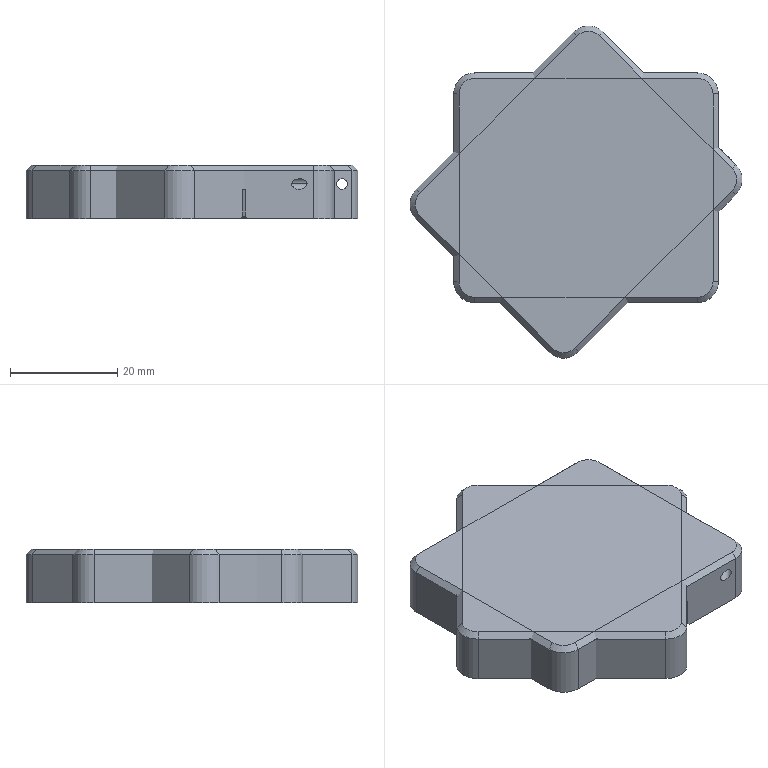NC program | NX | posted with a generic post | part box 61.954 x 61.954 x 10 mm
Lines 1 to 1285 of 3041:
N10 G17 G21 G94 G90
(PLANAR_MILL_5 , TOOL : D50面刀)
N12 T01 M6
N14 G54
N16 G17 G0 G90 X2.65 Y-96.458 B0. C0. S3500 M3
N18 G43 Z30. H1
N20 Z3.
N22 G94 G1 Z0. F800.
N24 Y-46.458
N26 Y41.158
N28 Y91.158
N30 Z3.
N32 G0 Z30.
N34 M5
(ADAPTIVE_MILLING , TOOL : D12开粗)
N36 T02 M6
N38 G54
N40 G17 G0 G90 X45.864 Y7.918 B0. C0. S5500 M3
N42 G43 Z30. H2
N44 Z-9.
N46 G94 G1 X45.758 Y7.813 Z-9.937 F2000.
N48 X45.652 Y7.707 Z-10.308
N50 X45.545 Y7.601 Z-10.58
N52 X45.439 Y7.495 Z-10.8
N54 X45.332 Y7.389 Z-10.984
N56 X45.226 Y7.284 Z-11.142
N58 X45.12 Y7.178 Z-11.28
N60 X45.013 Y7.072 Z-11.4
N62 X44.907 Y6.966 Z-11.505
N64 X44.801 Y6.861 Z-11.598
N66 X44.694 Y6.755 Z-11.679
N68 X44.588 Y6.649 Z-11.75
N70 X44.482 Y6.543 Z-11.81
N72 X44.375 Y6.437 Z-11.862
N74 X44.269 Y6.332 Z-11.905
N76 X44.163 Y6.226 Z-11.939
N78 X44.056 Y6.12 Z-11.966
N80 X43.95 Y6.014 Z-11.985
N82 X43.843 Y5.909 Z-11.996
N84 X43.737 Y5.803 Z-12.
N86 X42.422 Y4.495
N88 G3 X42.184 Y3.112 R1.212
N90 X44.131 Y0.105 R12.601
N92 G2 X45.422 Y-4.633 R6.785
N94 X43.61 Y-9.828 R11.92
N96 X39.648 Y-14.899 R33.153
N98 X31.725 Y-23.034 R288.997
N100 G1 X28.018 Y-26.746
N102 X11.27 Y-43.493
N104 G2 X6.905 Y-45.205 R6.347
N106 X1.737 Y-43.849 R10.676
N108 X-3.181 Y-40.307 R26.17
N110 X-10.332 Y-33.463 R170.745
N112 G1 X-15.854 Y-27.953
N114 X-40.717 Y-3.089
N116 G2 X-42.383 Y1.368 R6.391
N118 X-40.922 Y6.585 R10.897
N120 X-37.309 Y11.506 R27.426
N122 X-29.915 Y19.19 R197.683
N124 G1 X-24.963 Y24.151
N126 X-8.431 Y40.682
N128 G2 X-4.051 Y42.378 R6.371
N130 X1.113 Y41.008 R10.71
N132 X6.085 Y37.411 R26.458
N134 X13.286 Y30.51 R176.153
N136 G1 X19.337 Y24.47
N138 X38.705 Y5.1
N140 G2 X41.867 Y1.252 R35.803
N142 X43.105 Y-5.808 R9.477
N144 X40.632 Y-11.485 R15.987
N146 X36.045 Y-17.112 R45.201
N148 X27.401 Y-25.946 R391.348
N150 G1 X12.916 Y-40.434
N152 G2 X5.632 Y-42.863 R8.751
N154 X-0.237 Y-40.695 R14.363
N156 X-5.656 Y-36.475 R37.421
N158 X-15.223 Y-27.165 R313.101
N160 G1 X-19.574 Y-22.819
N162 X-37.671 Y-4.72
N164 G2 X-40.044 Y2.441 R8.75
N166 X-37.976 Y8.19 R14.179
N168 X-33.635 Y13.804 R36.949
N170 X-25.502 Y22.191 R267.646
N172 G1 X-21.794 Y25.904
N174 X-9.978 Y37.718
N176 G2 X-2.791 Y40.033 R8.762
N178 X2.946 Y37.939 R14.271
N180 X8.488 Y33.644 R36.929
N182 X17.577 Y24.812 R290.323
N184 G1 X21.662 Y20.73
N186 X36.143 Y6.246
N188 G2 X39.473 Y2.465 R34.167
N190 X41.128 Y-6.127 R10.742
N192 X38.425 Y-12.188 R17.777
N194 X33.354 Y-18.384 R50.057
N196 X23.832 Y-28.099 R439.795
N198 G1 X14.435 Y-37.499
N200 G2 X9.94 Y-40.443 R10.989
N202 X3.006 Y-40.323 R11.274
N204 X-2.733 Y-37.26 R20.291
N206 X-8.873 Y-31.967 R63.932
N208 X-20.486 Y-20.491 R824.186
N210 G1 X-34.684 Y-6.293
N212 G2 X-37.66 Y-1.679 R10.928
N214 X-37.454 Y5.255 R11.359
N216 X-34.31 Y11.033 R20.865
N218 X-28.513 Y17.668 R70.416
N220 X-17.842 Y28.442 R844.161
N222 X-10.805 Y35.444 R529.662
N224 X-1.961 Y37.933 R10.223
N226 X4.036 Y35.471 R16.616
N228 X9.946 Y30.78 R43.622
N230 X20.039 Y20.935 R364.834
N232 G1 X24.071 Y16.906
N234 X34.577 Y6.392
N236 G2 X37.549 Y2.972 R27.873
N238 X39.23 Y-6.569 R11.678
N240 X36.346 Y-12.812 R19.439
N242 X31.089 Y-19.22 R53.764
N244 X20.592 Y-29.925 R473.19
N246 X14.471 Y-36.003 R337.67
N248 X4.767 Y-38.917 R11.239
N250 G3 X3.796 Y-39.025 R5.737
N252 G1 X2.351
N254 X0.92 Y-38.819
N256 X-0.467 Y-38.412
N258 X-1.781 Y-37.811
N260 X-2.997 Y-37.029
N262 X-4.089 Y-36.083
N264 X-33.434 Y-6.738
N266 X-34.381 Y-5.646
N268 X-35.162 Y-4.43
N270 G2 X-35.968 Y-2.472 R12.133
N272 X-35.784 Y5.083 R12.762
N274 X-32.538 Y11.24 R21.937
N276 X-26.946 Y17.775 R66.263
N278 X-16.167 Y28.701 R685.961
N280 X-11.466 Y33.337 R159.128
N282 X-1.321 Y35.968 R11.28
N284 X4.953 Y33.189 R18.55
N286 X11.178 Y28.145 R50.002
N288 X20.887 Y18.67 R394.863
N290 G1 X25.716 Y13.846
N292 G2 X33.521 Y6.01 R786.277
N294 X36.613 Y1.834 R17.3
N296 X37.842 Y-2.86 R11.908
N298 G1 X37.927 Y-3.449
N300 Y-4.896
N302 G2 X36.789 Y-9.095 R13.102
N304 X32.768 Y-15.549 R28.888
N306 X25.933 Y-23.096 R104.429
N308 X14.24 Y-34.842 R885.476
N310 X8.976 Y-37.183 R12.835
N312 G3 X7.928 Y-37.812 R6.691
N314 G1 X6.613 Y-38.412
N316 X5.226 Y-38.819
N318 X4.484 Y-38.926
N320 X5.226 Y-38.819
N322 X6.613 Y-38.412
N324 X7.928 Y-37.812
N326 G2 X10.815 Y-36.145 R28.519
N328 G3 X15.297 Y-32.767 R24.971
N330 X20.577 Y-27.655 R178.112
N332 G1 X30.172 Y-18.052
N334 G3 X33.651 Y-13.275 R153.51
N336 G1 X34.722 Y-11.599
N338 G3 X35.932 Y-10.243 R25.584
N340 G1 X36.713 Y-9.028
N342 X37.314 Y-7.713
N344 X37.721 Y-6.326
N346 X37.314 Y-7.713
N348 X36.713 Y-9.028
N350 X35.932 Y-10.243
N352 G2 X34.722 Y-11.599 R25.584
N354 G3 X31.911 Y-14.459 R71.112
N356 G2 X25.581 Y-21.207 R123.303
N358 G1 X15.568 Y-31.237
N360 G2 X13.077 Y-33.244 R60.098
N362 G1 X10.237 Y-36.084
N364 G2 X8.955 Y-37.152 R12.357
N366 G3 X10.237 Y-36.084 R12.357
N368 G1 X34.986 Y-11.335
N370 X35.932 Y-10.243
N372 X36.713 Y-9.028
N374 X37.314 Y-7.713
N376 X37.721 Y-6.326
N378 X37.927 Y-4.896
N380 Y-3.449
N382 X37.722 Y-2.02
N384 X37.315 Y-0.633
N386 X36.714 Y0.682
N388 G3 X32.512 Y6.063 R32.571
N390 X24.435 Y14.277 R397.413
N392 G1 X13.008 Y25.684
N394 G3 X7.413 Y30.564 R117.001
N396 X4.55 Y33.282 R35.895
N398 G1 X3.334 Y34.063
N400 X2.019 Y34.664
N402 X0.632 Y35.071
N404 G3 X-3.491 Y35.413 R21.287
N406 X-10.19 Y33.039 R12.494
N408 X-15.143 Y28.802 R41.357
N410 G1 X-19.309 Y24.695
N412 X-29.488 Y14.51
N414 G3 X-32.611 Y9.971 R131.686
N416 X-34.479 Y6.34 R23.84
N418 G1 X-35.161 Y5.28
N420 X-35.762 Y3.965
N422 X-36.169 Y2.579
N424 X-36.375 Y1.148
N426 Y-0.297
N428 X-36.169 Y-1.728
N430 X-36.375 Y-0.297
N432 Y1.148
N434 X-36.169 Y2.579
N436 X-35.762 Y3.965
N438 X-35.161 Y5.28
N440 X-34.379 Y6.496
N442 G3 X-30.426 Y11.507 R66.
N444 G2 X-25.003 Y17.528 R72.996
N446 X-13.973 Y28.611 R992.035
N448 X-9.717 Y31.882 R30.303
N450 G1 X-8.333 Y32.641
N452 X-7.592 Y33.283
N454 X-6.376 Y34.064
N456 X-5.061 Y34.665
N458 X-3.674 Y35.072
N460 X-2.244 Y35.277
N462 X-0.798
N464 X-2.244
N466 X-3.674 Y35.072
N468 X-5.061 Y34.665
N470 X-6.376 Y34.064
N472 X-7.592 Y33.283
N474 G2 X-12.244 Y29.273 R504.034
N476 G3 X-19.165 Y22.563 R198.313
N478 G1 X-27.806 Y13.915
N480 X-30.109 Y10.912
N482 X-33.433 Y7.588
N484 X-8.685 Y32.336
N486 X-7.592 Y33.283
N488 X-6.376 Y34.064
N490 X-5.061 Y34.665
N492 X-3.674 Y35.072
N494 X-2.244 Y35.277
N496 X-0.798
N498 X0.632 Y35.071
N500 X2.019 Y34.664
N502 X3.334 Y34.063
N504 X4.55 Y33.282
N506 G2 X7.413 Y30.564 R35.895
N508 G1 X34.986 Y2.991
N510 X35.933 Y1.898
N512 G3 X37.991 Y3.023 R1.2
N514 G1 X37.868 Y3.322 Z-11.986
N516 X37.727 Y3.613 Z-11.973
N518 X36.988 Y5.163 Z-11.9
N520 X36.168 Y6.886 F15000.
N522 X36.064 Y7.061
N524 X35.933 Y7.218
N526 X7.717 Y35.434
N528 G3 X5.363 Y37.165 R9.703
N530 X1.49 Y38.546 R15.232
N532 X-1.233 Y38.895 R15.249
N534 X-3.186 Y38.768 R11.294
N536 X-4.871 Y38.466 R19.01
N538 X-8.004 Y37.174 R11.238
N540 X-11.524 Y34.523 R21.466
N542 G1 X-36.548 Y11.28
N544 G3 X-39.506 Y5.358 R9.424
N546 G1 X-39.875 Y1.842
N548 G3 X-39.351 Y0.72 R1.203
N550 G1 X-37.431 Y-0.661 Z-12. F2000.
N552 X-36.564 Y-1.284
N554 G2 X-36.113 Y-1.921 R1.206
N556 G1 X-35.762 Y-3.115
N558 G2 X-36.22 Y-4.442 R1.212
N560 G1 X-37.868 Y-5.62
N562 X-37.99 Y-5.707 Z-11.996
N564 X-38.112 Y-5.794 Z-11.985
N566 X-38.234 Y-5.882 Z-11.966
N568 X-38.356 Y-5.969 Z-11.939
N570 X-38.478 Y-6.056 Z-11.905
N572 X-38.6 Y-6.143 Z-11.862
N574 X-38.722 Y-6.231 Z-11.81
N576 X-38.844 Y-6.318 Z-11.75
N578 X-38.966 Y-6.405 Z-11.679
N580 X-39.088 Y-6.492 Z-11.598
N582 X-39.21 Y-6.58 Z-11.505
N584 X-39.332 Y-6.667 Z-11.4
N586 X-39.454 Y-6.754 Z-11.28
N588 X-39.576 Y-6.841 Z-11.142
N590 X-39.698 Y-6.929 Z-10.984
N592 X-39.82 Y-7.016 Z-10.8
N594 X-39.942 Y-7.103 Z-10.58
N596 X-40.064 Y-7.19 Z-10.308
N598 X-40.186 Y-7.278 Z-9.937
N600 X-40.308 Y-7.365 Z-9.
N602 G0 Z30.
N604 X17.764 Y28.59
N606 Z-2.299
N608 G1 X17.675 Y28.469 Z-3.236
N610 X17.586 Y28.349 Z-3.607
N612 X17.496 Y28.228 Z-3.879
N614 X17.407 Y28.108 Z-4.099
N616 X17.318 Y27.987 Z-4.283
N618 X17.228 Y27.867 Z-4.441
N620 X17.139 Y27.746 Z-4.579
N622 X17.049 Y27.626 Z-4.699
N624 X16.96 Y27.505 Z-4.804
N626 X16.871 Y27.385 Z-4.897
N628 X16.781 Y27.264 Z-4.978
N630 X16.692 Y27.144 Z-5.049
N632 X16.603 Y27.023 Z-5.109
N634 X16.513 Y26.903 Z-5.161
N636 X16.424 Y26.782 Z-5.204
N638 X16.335 Y26.662 Z-5.238
N640 X16.245 Y26.541 Z-5.265
N642 X16.156 Y26.421 Z-5.284
N644 X16.067 Y26.3 Z-5.295
N646 X15.977 Y26.18 Z-5.299
N648 X14.794 Y24.584
N650 G3 X14.83 Y23.093 R1.212
N652 G2 X15.676 Y21.855 R4.614
N654 G3 X18.447 Y18.34 R24.192
N656 X22.883 Y13.72 R169.017
N658 G1 X23.232 Y13.522
N660 X24.031 Y13.279
N662 X25.103 Y12.706
N664 X25.798 Y12.135
N666 X25.103 Y12.706
N668 X24.031 Y13.279
N670 G2 X22.838 Y13.682 R6.733
N672 X19.909 Y16.077 R16.483
N674 X16.369 Y20.027 R32.455
N676 X15.93 Y21.378 R11.695
N678 G1 X15.648 Y21.907
N680 X15.93 Y21.378
N682 G2 X16.4 Y19.725 R32.871
N684 G3 X18.265 Y16.767 R10.703
N686 X21.238 Y13.913 R16.259
N688 X21.69 Y13.749 R2.53
N690 G1 X22.868 Y13.632
N692 X23.155 Y13.545
N694 X22.868 Y13.632
N696 X21.509 Y13.762
N698 G2 X19.624 Y14.863 R5.435
N700 X16.481 Y18.68 R12.072
N702 X16.387 Y19.16 R2.728
N704 G1 X16.284 Y20.205
N706 G2 X16.422 Y18.518 R45.121
N708 G3 X17.904 Y15.716 R6.692
N710 X20.237 Y13.753 R7.366
N712 X20.751 Y13.663 R2.06
N714 G1 X21.659 Y13.752
N716 X20.527 Y13.645
N718 G2 X18.769 Y14.471 R3.705
N720 X16.341 Y17.786 R6.934
N722 X16.393 Y18.918 R4.218
N724 G3 X16.302 Y17.432 R7.494
N726 X18.067 Y14.405 R5.347
N728 X19.575 Y13.506 R3.537
N730 X20.449 Y13.633 R1.732
N732 G1 X20.673 Y13.655
N734 G3 X19.806 Y13.451 R4.907
N736 G2 X18.201 Y14.035 R2.725
N738 X16.152 Y17.027 R4.941
N740 X16.282 Y17.796 R1.819
N742 G3 X16.34 Y15.655 R2.573
N744 X18.688 Y13.321 R4.291
N746 X19.355 Y13.301 R1.488
N748 G1 X20.001 Y13.497
N750 X19.141 Y13.241
N752 G2 X17.686 Y13.684 R2.253
N754 X15.924 Y16.376 R3.91
N756 X16.112 Y17.236 R2.439
N758 G3 X15.836 Y16.236 R5.104
N760 X17.222 Y13.562 R3.388
N762 X18.541 Y13.024 R2.154
N764 X19.286 Y13.28 R1.632
N766 G2 X18.455 Y12.966 R1.734
N768 X16.531 Y13.965 R2.763
N770 X15.685 Y15.946 R2.989
N772 X15.929 Y16.633 R1.643
N774 G3 X15.586 Y15.863 R2.49
N776 X16.613 Y13.419 R2.907
N778 X18.011 Y12.763 R2.244
N780 X18.993 Y13.124 R2.099
N782 G2 X18.186 Y12.729 R5.901
N784 X16.567 Y13.256 R2.14
N786 X15.426 Y15.484 R2.835
N788 X15.719 Y16.24 R1.883
N790 G3 X15.326 Y15.433 R5.597
N792 X16.549 Y12.886 R2.701
N794 X17.943 Y12.581 R1.575
N796 G1 X18.151 Y12.667
N798 G3 X18.548 Y14.481 R1.32
N800 G1 X17.715 Y15.795
N802 G3 X15.436 Y15.711 R1.32
N804 X15.322 Y13.98 R1.852
N806 X17.09 Y12.341 R2.567
N808 X18.019 Y12.551 R1.318
N810 X18.279 Y14.418 R1.32
N812 G1 X17.422 Y15.53
N814 G3 X15.356 Y15.561 R1.32
N816 X15.016 Y14.318 R1.454
N818 X16.824 Y12.157 R2.54
N820 X17.82 Y12.384 R1.303
N822 G2 X18.478 Y12.849 R2.462
N824 G3 X17.643 Y12.246 R4.084
N826 G2 X16.426 Y12.192 R1.29
N828 X14.879 Y14.732 R2.514
N830 X15.295 Y15.486 R1.557
N832 G3 X14.803 Y14.827 R4.353
N834 X15.531 Y12.436 R2.329
N836 X16.879 Y11.884 R1.811
N838 X17.792 Y12.362 R1.578
N840 G2 X17.126 Y11.881 R3.209
N842 X15.487 Y12.301 R1.779
N844 X14.588 Y14.381 R2.364
N846 X15.002 Y15.13 R1.556
N848 G3 X14.481 Y14.33 R2.158
N850 X16.352 Y11.626 R2.31
N852 X17.257 Y11.92 R1.32
N854 X17.447 Y13.534 R1.32
N856 G1 X16.817 Y14.572
N858 G3 X14.669 Y14.724 R1.32
N860 X14.329 Y13.218 R1.579
N862 X16.111 Y11.438 R2.305
N864 X17.274 Y11.936 R1.337
N866 G1 X17.448 Y12.079
N868 G2 X16.797 Y11.508 R15.63
N870 X15.426 Y11.571 R1.467
N872 X14.172 Y13.93 R2.314
N874 X14.585 Y14.622 R1.39
N876 G3 X14.056 Y12.887 R1.567
N878 X15.909 Y11.171 R2.271
N880 X17.037 Y11.7 R1.37
N882 G2 X16.473 Y11.211 R2.825
N884 X14.811 Y11.514 R1.703
N886 X13.893 Y13.68 R2.238
N888 X14.329 Y14.366 R1.435
N890 G3 X13.745 Y13.53 R1.691
N892 X15.696 Y10.9 R2.249
N894 X16.775 Y11.438 R1.391
N896 G2 X16.212 Y10.946 R2.963
N898 X14.552 Y11.23 R1.708
N900 X13.602 Y13.368 R2.229
N902 X14.05 Y14.087 R1.426
N904 G3 X13.482 Y13.318 R1.765
N906 X15.416 Y10.631 R2.246
N908 X16.51 Y11.173 R1.397
N910 G2 X15.949 Y10.68 R3.084
N912 X14.426 Y10.86 R1.654
N914 X13.307 Y13.022 R2.282
N916 X13.766 Y13.803 R1.395
N918 G3 X13.202 Y13.073 R2.01
N920 X15.168 Y10.358 R2.251
N922 X16.281 Y10.944 R1.505
N924 G2 X15.664 Y10.401 R3.089
N926 X14.151 Y10.587 R1.665
N928 X13.036 Y12.779 R2.246
N930 X13.497 Y13.534 R1.417
N932 G3 X12.906 Y12.707 R1.751
N934 X14.87 Y10.087 R2.262
N936 X15.966 Y10.629 R1.398
N938 G2 X15.405 Y10.136 R3.101
N940 X13.699 Y10.432 R1.745
N942 X12.771 Y12.55 R2.188
N944 X13.21 Y13.247 R1.43
N946 G3 X12.623 Y12.403 R1.686
N948 X14.622 Y9.811 R2.256
N950 X15.733 Y10.396 R1.504
N952 G2 X15.116 Y9.854 R3.081
N954 X13.432 Y10.151 R1.749
N956 X12.486 Y12.233 R2.215
N958 X12.896 Y12.933 R1.381
N960 G3 X12.399 Y11.195 R1.527
N962 X14.341 Y9.536 R2.261
N964 X15.46 Y10.123 R1.506
N966 G2 X14.844 Y9.58 R3.129
N968 X13.164 Y9.871 R1.746
N970 X12.217 Y11.979 R2.203
N972 X12.669 Y12.706 R1.426
N974 G3 X12.081 Y11.882 R1.742
N976 X14.042 Y9.262 R2.263
N978 X15.143 Y9.806 R1.4
N980 G2 X14.582 Y9.312 R3.142
N982 X13.214 Y9.401 R1.565
N984 X11.918 Y11.617 R2.292
N986 X12.389 Y12.426 R1.395
N988 G3 X11.804 Y11.603 R1.712
N990 X13.779 Y8.985 R2.267
N992 X14.86 Y9.523 R1.392
N994 G2 X14.298 Y9.032 R2.987
N996 X12.609 Y9.326 R1.74
N998 X11.643 Y11.338 R2.272
N1000 X12.116 Y12.153 R1.395
N1002 G3 X11.529 Y11.323 R1.714
N1004 X13.5 Y8.712 R2.267
N1006 X14.642 Y9.305 R1.512
N1008 G2 X14.027 Y8.759 R3.289
N1010 X12.339 Y9.047 R1.738
N1012 X11.389 Y11.148 R2.201
N1014 X11.843 Y11.881 R1.425
N1016 G3 X11.256 Y11.051 R1.721
N1018 X13.242 Y8.44 R2.255
N1020 X14.365 Y9.028 R1.507
N1022 G2 X13.749 Y8.485 R3.148
N1024 X12.053 Y8.783 R1.748
N1026 X11.121 Y10.899 R2.187
N1028 X11.562 Y11.599 R1.429
N1030 G3 X10.974 Y10.753 R1.689
N1032 X12.973 Y8.164 R2.258
N1034 X14.086 Y8.749 R1.505
N1036 G2 X13.469 Y8.207 R3.09
N1038 X11.782 Y8.504 R1.75
N1040 X10.837 Y10.584 R2.213
N1042 X11.247 Y11.284 R1.381
N1044 G3 X10.75 Y9.546 R1.526
N1046 X12.7 Y7.889 R2.256
N1048 X13.811 Y8.474 R1.504
N1050 G2 X13.182 Y7.926 R2.931
N1052 X11.493 Y8.24 R1.769
N1054 X10.564 Y10.325 R2.21
N1056 X11.018 Y11.055 R1.426
N1058 G3 X10.471 Y10.381 R2.069
N1060 X11.47 Y7.941 R2.211
N1062 X12.98 Y7.73 R1.564
N1064 X13.483 Y8.146 R1.51
N1066 G2 X11.92 Y7.612 R1.309
N1068 X10.28 Y10.051 R2.285
N1070 X10.795 Y10.832 R1.344
N1072 G3 X10.153 Y10.02 R1.491
N1074 X12.277 Y7.322 R2.275
N1076 X13.377 Y8.016 R1.486
N1078 G2 X12.815 Y7.416 R3.065
N1080 X11.299 Y7.463 R1.63
N1082 X10.003 Y9.85 R2.292
N1084 X10.492 Y10.584 R1.344
N1086 G3 X9.837 Y9.032 R1.452
N1088 X12.011 Y7.025 R2.353
N1090 X13.134 Y7.721 R1.48
N1092 G2 X12.573 Y7.121 R3.079
N1094 X11.059 Y7.158 R1.654
N1096 X9.717 Y9.619 R2.343
N1098 X10.209 Y10.351 R1.347
N1100 G3 X9.545 Y8.738 R1.495
N1102 X11.812 Y6.728 R2.37
N1104 X12.713 Y7.207 R1.297
N1106 X12.666 Y8.52 R1.321
N1108 G1 X11.877 Y9.79
N1110 G3 X9.919 Y10.114 R1.32
N1112 X9.349 Y8.726 R1.454
N1114 X11.614 Y6.502 R2.411
N1116 X12.627 Y7.059 R1.28
N1118 X12.486 Y8.68 R1.32
N1120 G1 X11.442 Y9.798
N1122 G3 X9.855 Y10.061 R1.32
N1124 X9.165 Y8.928 R1.328
N1126 X11.502 Y6.272 R2.455
N1128 X12.54 Y6.885 R1.28
N1130 G2 X12.856 Y7.381 R2.147
N1132 G3 X12.429 Y6.689 R3.579
N1134 G2 X11.23 Y6.197 R1.284
N1136 X9.109 Y9.297 R2.476
N1138 X9.839 Y10.052 R1.353
N1140 G3 X9.043 Y9.433 R1.697
N1142 X9.299 Y7.029 R2.309
N1144 X11.524 Y5.966 R2.389
N1146 X12.539 Y6.882 R1.471
N1148 G2 X12.106 Y6.183 R3.148
N1150 X10.596 Y5.932 R1.639
N1152 X8.765 Y9.107 R2.605
N1154 X9.499 Y9.871 R1.353
N1156 G3 X8.706 Y9.259 R1.715
N1158 X8.949 Y6.758 R2.393
N1160 X11.37 Y5.626 R2.515
N1162 X12.354 Y6.537 R1.485
N1164 G2 X11.919 Y5.834 R3.143
N1166 X10.222 Y5.614 R1.785
N1168 X8.405 Y8.895 R2.726
N1170 X9.157 Y9.688 R1.354
N1172 G3 X8.404 Y9.144 R1.829
N1174 X8.43 Y6.732 R2.378
N1176 X11.165 Y5.254 R2.736
N1178 X12.107 Y6.034 R1.279
N1180 X11.808 Y7.392 R1.321
N1182 G1 X10.104 Y9.143
N1184 G3 X8.783 Y9.488 R1.321
N1186 X7.977 Y8.599 R1.275
N1188 X9.227 Y5.406 R2.87
N1190 X11.381 Y5.082 R2.358
N1192 X12.14 Y6.136 R1.421
N1194 G2 X11.853 Y5.379 R2.984
N1196 X10.431 Y4.841 R1.645
N1198 X7.795 Y8.509 R2.973
N1200 X8.615 Y9.438 R1.35
N1202 X10. Y9.026 R1.32
N1204 G1 X11.756 Y6.954
N1206 G2 X12.012 Y5.717 R1.321
N1208 X11.093 Y4.813 R1.232
N1210 X8.414 Y5.638 R2.733
N1212 X7.712 Y8.708 R2.891
N1214 X8.783 Y9.488 R1.466
N1216 G3 X7.93 Y9.164 R2.71
N1218 X7.293 Y7.297 R2.126
N1220 X10.557 Y4.426 R3.178
N1222 X11.995 Y5.658 R1.45
N1224 G2 X11.707 Y4.889 R3.119
N1226 X10.059 Y4.297 R1.917
N1228 X7.14 Y7.974 R3.266
N1230 X7.964 Y9.229 R1.607
N1232 G1 X8.272 Y9.334
N1234 G3 X7.41 Y8.925 R1.789
N1236 X6.907 Y6.708 R2.487
N1238 X10.423 Y3.982 R3.392
N1240 X11.742 Y4.834 R1.485
N1242 G1 X11.769 Y4.904
N1244 G3 X11.501 Y6.033 R1.321
N1246 G1 X9.244 Y8.778
N1248 G3 X7.841 Y9.203 R1.32
N1250 X6.722 Y8.082 R1.605
N1252 X7.743 Y4.575 R3.374
N1254 X10.787 Y3.74 R3.232
N1256 X11.768 Y4.79 R1.306
N1258 X11.439 Y5.794 R1.322
N1260 G1 X8.834 Y8.715
N1262 G3 X7.62 Y9.136 R1.321
N1264 X6.585 Y8.277 R1.494
N1266 X6.867 Y5.048 R3.274
N1268 X10.386 Y3.323 R3.636
N1270 X11.625 Y4.127 R1.596
N1272 X11.786 Y4.973 R2.23
N1274 G1 X11.874 Y5.26
N1276 G3 X11.71 Y4.261 R4.087
N1278 G2 X10.825 Y3.332 R1.392
N1280 X7.905 Y3.713 R3.238
N1282 X6.13 Y7.482 R3.793
N1284 X6.923 Y8.913 R2.211
N1286 X7.405 Y9.112 R2.037
N1288 X8.609 Y8.668 R1.321
N1290 G1 X11.418 Y5.399
N1292 G2 X11.731 Y4.409 R1.322
N1294 X11.026 Y3.325 R1.293
N1296 X8.265 Y3.29 R3.069
N1298 X5.922 Y7.426 R3.935
N1300 X6.713 Y8.892 R2.242
N1302 X7.62 Y9.136 R1.683
N1304 G3 X6.627 Y8.955 R2.768
N1306 X5.594 Y7.173 R2.444
N1308 X9.684 Y2.614 R4.124
N1310 X11.378 Y3.262 R2.424
N1312 X11.718 Y4.284 R1.553
N1314 G2 X11.615 Y3.543 R6.324
N1316 X10.431 Y2.589 R1.864
N1318 X6.919 Y3.397 R3.802
N1320 X5.442 Y7.469 R4.136
N1322 X6.272 Y8.851 R2.387
N1324 X7.009 Y9.076 R1.473
N1326 G3 X6.091 Y8.851 R1.841
N1328 X5.02 Y6.723 R2.764
N1330 X9.562 Y2.055 R4.46
N1332 X11.393 Y2.821 R2.631
N1334 X11.677 Y3.656 R1.344
N1336 X11.351 Y4.426 R1.326
N1338 G1 X7.681 Y8.591
N1340 G3 X6.561 Y9.032 R1.321
N1342 X5.347 Y8.382 R1.512
N1344 X4.801 Y5.212 R3.626
N1346 X9.562 Y1.655 R4.707
N1348 X11.458 Y2.512 R2.703
N1350 X11.71 Y3.328 R1.348
N1352 G1 X11.674 Y3.838
N1354 G2 X11.716 Y2.955 R13.676
N1356 X10.852 Y1.881 R1.679
N1358 X7.686 Y1.706 R3.789
N1360 X4.45 Y6.651 R4.854
N1362 X5.605 Y8.842 R2.999
N1364 X6.246 Y9.027 R1.475
N1366 X7.224 Y8.594 R1.322
N1368 G1 X7.53 Y8.256
N1370 X9.119 Y6.505 Z-5.199
N1372 X9.149 Y6.471 F15000.
N1374 X10.738 Y4.72 Z-5.299 F2000.
N1376 X11.381 Y4.012
N1378 G2 X11.717 Y3.254 R1.326
N1380 X11.261 Y2.054 R1.325
N1382 X8.624 Y1.267 R3.326
N1384 X4.215 Y6.668 R4.991
N1386 X5.358 Y8.838 R3.065
N1388 X6.41 Y9.017 R1.43
N1390 G3 X5.464 Y9.008 R2.143
N1392 X4.093 Y7.52 R2.537
N1394 X4.716 Y3.132 R4.762
N1396 X9.417 Y0.843 R5.119
N1398 X11.577 Y1.97 R3.056
N1400 X11.728 Y3.139 R1.692
N1402 G2 X11.776 Y2.317 R5.515
N1404 X10.636 Y1.027 R2.113
N1406 X6.805 Y1.039 R4.432
N1408 X3.595 Y6.548 R5.392
N1410 X4.935 Y8.903 R3.306
N1412 X5.949 Y9.063 R1.435
N1414 G3 X5.127 Y9.102 R3.999
N1416 X3.542 Y7.596 R2.628
N1418 X3.827 Y3.164 R4.996
N1420 X8.884 Y0.146 R5.659
N1422 X11.565 Y1.32 R3.618
N1424 X11.835 Y2.375 R1.289
N1426 X11.516 Y2.991 R1.332
N1428 G1 X10.549 Y4.042
N1430 X8.948 Y5.782 Z-5.199
N1432 X8.468 Y6.303 F15000.
N1434 X6.867 Y8.043 Z-5.299 F2000.
N1436 X6.516 Y8.43
N1438 X6.153 Y8.805
N1440 G3 X5.426 Y9.114 R1.327
N1442 X4.041 Y8.696 R1.615
N1444 X2.74 Y5.781 R3.933
N1446 X8.832 Y-0.326 R6.008
N1448 X11.485 Y0.729 R3.965
N1450 X11.935 Y2.062 R1.422
N1452 G1 X11.779 Y2.628
N1454 G2 X12.012 Y1.696 R11.41
N1456 X11.295 Y0.375 R1.893
N1458 X8.023 Y-0.55 R4.354
N1460 X2.467 Y5.754 R6.209
N1462 X3.741 Y8.693 R4.159
N1464 X5.024 Y9.177 R1.615
N1466 G1 X5.098 Y9.166
N1468 G2 X5.743 Y8.789 R1.329
N1470 G1 X6.53 Y7.954
N1472 X8.151 Y6.232 Z-5.199
N1474 X8.873 Y5.466 F15000.
N1476 X10.494 Y3.744 Z-5.299 F2000.
N1478 X11.655 Y2.512
N1480 G2 X11.957 Y1.99 R1.341
N1482 X11.783 Y0.771 R1.329
N1484 X9.448 Y-0.714 R3.54
N1486 X4.322 Y0.806 R5.963
N1488 X2.269 Y6.418 R6.177
N1490 X3.716 Y8.925 R3.983
N1492 X5.201 Y9.136 R1.444
N1494 G3 X4.253 Y9.309 R2.089
N1496 X2.463 Y7.96 R2.806
N1498 X2.019 Y3.438 R5.446
N1500 X8.497 Y-1.317 R6.732
N1502 X11.589 Y-0.061 R4.446
N1504 X12.164 Y1.14 R1.753
N1506 X11.997 Y1.857 R2.778
N1508 G1 X12.207 Y1.099
N1510 G2 X11.56 Y-0.299 R2.05
N1512 X8.178 Y-1.584 R4.636
N1514 X1.446 Y5.542 R6.923
N1516 X2.908 Y8.831 R4.663
N1518 X4.234 Y9.394 R1.955
N1520 X4.743 Y9.275 R3.973
N1522 G3 X3.946 Y9.477 R4.312
N1524 X2.143 Y8.473 R2.697
N1526 X0.998 Y4.399 R5.344
N1528 X8.163 Y-2.105 R7.322
N1530 X11.708 Y-0.724 R4.939
N1532 X12.38 Y0.577 R2.151
N1534 X12.138 Y1.391 R1.486
N1536 G2 X12.436 Y0.586 R1.658
N1538 X11.522 Y-1.142 R2.547
N1540 X7.723 Y-2.378 R5.272
N1542 X0.663 Y5.243 R7.525
N1544 X2.249 Y8.909 R5.114
N1546 X3.561 Y9.557 R2.372
N1548 X4.007 Y9.505 R5.03
N1550 X4.547 Y8.972 R1.206
N1552 G1 X4.943 Y8.194
N1554 X6.016 Y6.087 Z-5.199
N1556 X6.492 Y5.153 F15000.
N1558 X6.573 Y5.021
N1560 X6.667 Y4.897
N1562 X7.689 Y3.754
N1564 G3 X8.044 Y3.482 R1.272
N1566 G1 X8.757 Y3.123
N1568 X10.869 Y2.058 Z-5.299 F2000.
N1570 X11.391 Y1.799
N1572 X11.906 Y1.526
N1574 G2 X12.297 Y1.094 R1.218
N1576 X12.373 Y-0.147 R1.377
N1578 X10.292 Y-2.184 R3.739
N1580 X5.095 Y-2.074 R6.565
N1582 X0.352 Y5.179 R7.762
N1584 X1.856 Y8.868 R5.393
N1586 X3.364 Y9.659 R2.507
N1588 X3.878 Y9.568 R2.
N1590 X4.489 Y8.994 R1.204
N1592 G1 X4.874 Y8.216
N1594 X5.923 Y6.097 Z-5.199
N1596 X6.349 Y5.237 F15000.
N1598 X6.435 Y5.093
N1600 X6.538 Y4.961
N1602 X7.76 Y3.622
N1604 G3 X8.105 Y3.359 R1.283
N1606 G1 X8.766 Y3.025
N1608 X10.877 Y1.959 Z-5.299 F2000.
N1610 X11.431 Y1.683
N1612 X11.977 Y1.393
N1614 G2 X12.368 Y0.961 R1.218
N1616 X12.457 Y-0.222 R1.429
N1618 X10.639 Y-2.272 R3.64
N1620 X5.627 Y-2.609 R6.452
N1622 X0.034 Y5.028 R8.012
N1624 X1.584 Y8.945 R5.634
N1626 X3.128 Y9.768 R2.677
N1628 X4.038 Y9.49 R1.563
N1630 G1 X4.253 Y9.424
N1632 G2 X3.462 Y9.793 R3.73
N1634 G3 X2.054 Y9.619 R1.801
N1636 X-0.075 Y7.061 R4.588
N1638 X0.389 Y1.151 R7.451
N1640 X7.781 Y-3.511 R8.361
N1642 X11.836 Y-1.966 R5.795
N1644 X12.782 Y-0.214 R3.097
N1646 X12.669 Y0.397 R1.569
N1648 G1 X12.422 Y0.861
N1650 X12.801 Y0.113
N1652 G2 X12.385 Y-1.573 R2.296
N1654 X9.283 Y-3.618 R5.085
N1656 X2.972 Y-2.321 R7.911
N1658 X-0.795 Y5.164 R8.559
N1660 X0.925 Y9.112 R5.941
N1662 X2.801 Y10.001 R2.954
N1664 X3.573 Y9.738 R1.628
N1666 G3 X2.831 Y10.094 R4.793
N1668 X0.789 Y9.436 R2.794
N1670 X-1.256 Y5.716 R5.808
N1672 X1.362 Y-1.774 R8.748
N1674 X8.634 Y-4.313 R8.692
N1676 X12.388 Y-2.317 R5.85
N1678 X13.112 Y-0.553 R2.894
N1680 X12.711 Y0.319 R1.407
N1682 G2 X13.165 Y-0.466 R1.544
N1684 X12.487 Y-2.509 R2.896
N1686 X8.868 Y-4.582 R5.872
N1688 X1.829 Y-2.669 R8.783
N1690 X-1.67 Y5.004 R9.195
N1692 X0.095 Y9.175 R6.479
N1694 X2.25 Y10.268 R3.543
N1696 X2.898 Y10.108 R1.515
N1698 X3.445 Y9.105 R1.201
N1700 X3.313 Y8.543 Z-5.274 R1.388
N1702 G1 X2.637 Y6.893 Z-5.199
N1704 X2.48 Y6.516 F15000.
N1706 X2.337 Y6.134
N1708 G3 X2.898 Y4.787 R1.2
N1710 X3.41 Y4.543 R2.014
N1712 X4.809 Y6.19 R1.205
N1714 G1 X4.006 Y8.414 Z-5.299 F2000.
N1716 X3.817 Y8.945
N1718 X3.614 Y9.47
N1720 G3 X3.11 Y9.986 R1.208
N1722 G2 X2.728 Y10.244 R7.214
N1724 G3 X1.172 Y10.244 R2.036
N1726 X-1.363 Y7.935 R4.839
N1728 X-1.904 Y1.853 R8.098
N1730 X7.169 Y-5.31 R9.856
N1732 X12.104 Y-3.635 R7.114
N1734 X13.49 Y-1.153 R3.932
N1736 X13.246 Y-0.333 R1.347
N1738 G1 X12.913 Y0.073
N1740 G2 X13.46 Y-0.64 R7.066
N1742 X13.304 Y-2.365 R2.316
N1744 X10.533 Y-4.97 R5.388
N1746 X4.039 Y-5.054 R8.597
N1748 X-2.598 Y3.95 R10.147
N1750 X-1.019 Y8.977 R7.433
N1752 X1.537 Y10.544 R4.224
N1754 X2.881 Y10.133 R1.459
N1756 G3 X2.221 Y10.624 R4.376
N1758 X0.14 Y10.386 R2.766
N1760 X-2.553 Y7.353 R5.796
N1762 X-2.437 Y0.382 R9.156
N1764 X7.007 Y-6.263 R10.621
N1766 X12.244 Y-4.54 R7.822
N1768 X13.853 Y-1.972 R4.564
N1770 X13.482 Y-0.622 R1.374
N1772 G1 X13.292 Y-0.39
N1774 X13.819 Y-1.002
N1776 G2 X13.865 Y-2.538 R2.158
N1778 X11.602 Y-5.36 R5.21
N1780 X5.411 Y-6.461 R8.664
N1782 X-3.543 Y3.718 R10.933
N1784 X-1.956 Y9.014 R8.122
N1786 X0.944 Y10.887 R4.804
N1788 X2.504 Y10.442 R1.65
N1790 G3 X1.839 Y10.956 R14.361
N1792 X-0.382 Y10.793 R2.913
N1794 X-3.314 Y7.762 R6.114
N1796 X-3.603 Y0.601 R9.63
N1798 X6.596 Y-7.238 R11.469
N1800 X12.369 Y-5.501 R8.63
N1802 X14.274 Y-2.629 R5.136
N1804 X14.136 Y-1.317 R1.734
N1806 X13.584 Y-0.723 R5.636
N1808 G1 X14.21 Y-1.369
N1810 G2 X14.376 Y-2.875 R2.114
N1812 X12.435 Y-5.814 R5.228
N1814 X6.44 Y-7.595 R8.868
N1816 X-4.518 Y3.453 R11.741
N1818 X-2.794 Y9.234 R8.793
N1820 X0.21 Y11.242 R5.313
N1822 X1.597 Y11.169 R2.239
N1824 X2.027 Y10.833 R1.936
N1826 G3 X1.329 Y11.387 R1.946
N1828 X-1.096 Y11.159 R3.339
N1830 X-4.215 Y7.947 R6.63
N1832 X-4.724 Y0.711 R10.231
N1834 X6.434 Y-8.253 R12.328
N1836 X12.643 Y-6.385 R9.354
N1838 X14.735 Y-3.268 R5.614
N1840 X14.707 Y-1.969 R2.18
N1842 X14.07 Y-1.21 R2.724
N1844 G1 X14.695 Y-1.856
N1846 G2 X14.841 Y-3.573 R2.411
N1848 X12.705 Y-6.719 R5.779
N1850 X6.427 Y-8.628 R9.552
N1852 X-5.524 Y3.233 R12.604
N1854 X-3.716 Y9.411 R9.512
N1856 X-0.582 Y11.619 R5.937
N1858 X1.161 Y11.594 R2.78
N1860 X1.738 Y11.122 R2.056
N1862 G1 X1.144 Y11.693
N1864 G3 X-0.879 Y11.882 R2.871
N1866 X-4.344 Y9.454 R6.166
N1868 X-6.154 Y2.877 R10.
N1870 X6.486 Y-9.303 R13.173
N1872 X12.953 Y-7.284 R10.051
N1874 X15.218 Y-3.977 R6.214
N1876 X15.23 Y-2.517 R2.594
N1878 X14.996 Y-2.135 R3.506
N1880 G1 X14.518 Y-1.658
N1882 X15.197 Y-2.356
N1884 G2 X15.371 Y-4.117 R2.529
N1886 X13.18 Y-7.503 R6.145
N1888 X6.699 Y-9.69 R10.155
N1890 X-4.328 Y-3.651 R13.441
N1892 X-6.398 Y5.496 R12.639
N1894 X-3.698 Y10.675 R9.134
N1896 X-0.433 Y12.196 R5.485
N1898 X0.855 Y11.966 R2.172
N1900 X1.334 Y11.526 R5.999
N1902 G1 X0.686 Y12.15
N1904 G3 X-1.531 Y12.351 R3.088
N1906 X-5.149 Y9.876 R6.591
N1908 X-7.222 Y3.036 R10.599
N1910 X-0.668 Y-8.198 R14.01
N1912 X8.988 Y-10.141 R13.232
N1914 X14.483 Y-7.042 R9.593
N1916 X15.862 Y-3.727 R5.454
N1918 X15.529 Y-2.668 R1.454
N1920 G1 X15.052 Y-2.191
N1922 X15.731 Y-2.889
N1924 G2 X15.936 Y-4.633 R2.622
N1926 X13.831 Y-8.165 R6.409
N1928 X7.446 Y-10.738 R10.581
N1930 X-3.426 Y-6.515 R14.107
N1932 X-7.605 Y4.167 R14.011
N1934 X-5.023 Y10.57 R10.41
N1936 X-1.425 Y12.648 R6.434
N1938 X0.245 Y12.519 R3.086
N1940 X0.91 Y11.951 R2.446
N1942 G1 X0.27 Y12.583
N1944 G3 X-1.765 Y12.932 R2.96
N1946 X-5.547 Y10.81 R6.578
N1948 X-8.266 Y4.286 R10.761
N1950 X-4.381 Y-6.559 R14.514
N1952 X7.226 Y-11.45 R14.786
N1954 X13.619 Y-9.151 R11.221
N1956 X16.126 Y-4.72 R14.243
N1958 X16.104 Y-3.321 R1.769
N1960 X15.582 Y-2.722 R3.009
N1962 G2 X16.21 Y-3.497 R2.553
N1964 X16.111 Y-4.759 R1.529
N1966 G1 X15.566 Y-6.126
N1968 G2 X13.569 Y-9.226 R16.323
N1970 X10.468 Y-11.201 R7.147
N1972 X2.173 Y-11.22 R13.308
N1974 X-8.663 Y1.987 R15.479
N1976 X-6.878 Y9.707 R12.111
N1978 X-3.086 Y12.894 R8.017
N1980 X-0.393 Y13.08 R4.28
N1982 X0.35 Y12.51 R1.873
N1984 G3 X-0.391 Y13.187 R4.218
N1986 X-2.156 Y13.443 R2.516
N1988 X-6.331 Y11.083 R13.396
N1990 X-8.974 Y6.455 R9.573
N1992 X-8.128 Y-2.906 R14.332
N1994 X5.47 Y-12.557 R16.106
N1996 X10.66 Y-11.827 R12.308
N1998 X13.234 Y-9.578 R13.787
N2000 G2 X10.213 Y-12.102 R13.082
N2002 X6.566 Y-12.955 R8.573
N2004 X-3.518 Y-9.53 R15.619
N2006 X-9.822 Y2.739 R16.202
N2008 X-8.27 Y9.189 R12.231
N2010 X-6.043 Y11.324 R12.571
N2012 G3 X-8.27 Y9.189 R12.695
N2014 X-10.355 Y4.623 R8.203
N2016 X-8.758 Y-4.307 R15.136
N2018 X4.321 Y-13.585 R17.059
N2020 X6.917 Y-13.618 R11.419
N2022 G1 X7.728 Y-13.363
N2024 X9.409 Y-12.596
N2026 X10.24 Y-12.085
N2028 G2 X6.048 Y-13.841 R12.709
N2030 X1.419 Y-13.394 R11.097
N2032 X-10.782 Y0.723 R17.349
N2034 X-10.636 Y5.258 R13.021
N2036 X-9.333 Y7.753 R13.863
N2038 G1 X-9.967 Y6.721
N2040 G3 X-11.191 Y3.552 R16.169
N2042 X-11.124 Y-1.097 R10.468
N2044 X-4.109 Y-11.517 R17.611
N2046 X1.833 Y-14.257 R16.863
N2048 G1 X2.293 Y-14.29
N2050 G3 X5.961 Y-13.906 R16.323
N2052 G1 X6.536 Y-13.733
N2054 X5.802 Y-13.943
N2056 X3.977 Y-14.233
N2058 X2.25 Y-14.291
N2060 G2 X-0.551 Y-13.829 R11.027
N2062 X-7.075 Y-9.518 R16.321
N2064 X-11.592 Y-0.935 R17.4
N2066 G1 X-11.644 Y-0.159
N2068 G2 X-11.219 Y3.465 R16.259
N2070 G1 X-11.174 Y3.608
N2072 G3 X-11.565 Y1.506 R20.494
N2074 G1 X-11.646 Y-0.218
N2076 G3 X-11.095 Y-3.928 R16.359
N2078 X-9.631 Y-7.311 R16.133
N2080 X-7.41 Y-10.156 R16.05
N2082 X-3.168 Y-13.058 R15.351
N2084 X0.452 Y-14.125 R16.094
N2086 G1 X0.9 Y-14.168
N2088 X0.291 Y-14.099
N2090 G2 X-3.168 Y-13.058 R16.407
N2092 X-7.41 Y-10.156 R15.354
N2094 X-9.802 Y-7.006 R15.475
N2096 X-9.858 Y-5.953 R1.322
N2098 G1 X-9.277 Y-4.393
N2100 X-8.451 Y-2.178 Z-5.199
N2102 X-4.312 Y8.922 F15000.
N2104 X-3.486 Y11.138 Z-5.299 F2000.
N2106 X-2.913 Y12.675
N2108 G2 X-2.156 Y13.443 R1.322
N2110 X-0.392 Y13.252 R1.733
N2112 G1 X-0.18 Y13.04
N2114 G3 X-1.341 Y13.661 R1.595
N2116 X-1.969 Y13.516 R1.833
N2118 X-2.687 Y12.031 R1.212
N2120 G1 X-2.144 Y10.264
N2122 X-2.1 Y10.121 Z-5.295
N2124 X-2.056 Y9.977 Z-5.284
N2126 X-2.012 Y9.834 Z-5.265
N2128 X-1.968 Y9.691 Z-5.238
N2130 X-1.924 Y9.547 Z-5.204
N2132 X-1.879 Y9.404 Z-5.161
N2134 X-1.835 Y9.261 Z-5.109
N2136 X-1.791 Y9.117 Z-5.049
N2138 X-1.747 Y8.974 Z-4.978
N2140 X-1.703 Y8.83 Z-4.897
N2142 X-1.659 Y8.687 Z-4.804
N2144 X-1.615 Y8.544 Z-4.699
N2146 X-1.571 Y8.4 Z-4.579
N2148 X-1.527 Y8.257 Z-4.441
N2150 X-1.483 Y8.113 Z-4.283
N2152 X-1.439 Y7.97 Z-4.099
N2154 X-1.395 Y7.827 Z-3.879
N2156 X-1.351 Y7.683 Z-3.607
N2158 X-1.307 Y7.54 Z-3.236
N2160 X-1.263 Y7.397 Z-2.299
N2162 G0 Z30.
N2164 M5
(ADAPTIVE_MILLING_COPY , TOOL : D6精光)
N2166 T13 M6
N2168 G54
N2170 G17 G0 G90 X-1.295 Y12.102 B0. C0. S5500 M3
N2172 G43 Z30. H13
N2174 Z-2.299
N2176 G94 G1 X-1.204 Y12.221 Z-3.236 F2000.
N2178 X-1.113 Y12.341 Z-3.607
N2180 X-1.022 Y12.46 Z-3.879
N2182 X-0.93 Y12.579 Z-4.099
N2184 X-0.839 Y12.698 Z-4.283
N2186 X-0.748 Y12.817 Z-4.441
N2188 X-0.657 Y12.936 Z-4.579
N2190 X-0.566 Y13.055 Z-4.699
N2192 X-0.474 Y13.174 Z-4.804
N2194 X-0.383 Y13.293 Z-4.897
N2196 X-0.292 Y13.412 Z-4.978
N2198 X-0.201 Y13.531 Z-5.049
N2200 X-0.11 Y13.651 Z-5.109
N2202 X-0.018 Y13.77 Z-5.161
N2204 X0.073 Y13.889 Z-5.204
N2206 X0.164 Y14.008 Z-5.238
N2208 X0.255 Y14.127 Z-5.265
N2210 X0.346 Y14.246 Z-5.284
N2212 X0.438 Y14.365 Z-5.295
N2214 X0.529 Y14.484 Z-5.299
N2216 X1.112 Y15.246
N2218 G3 X1.06 Y16.043 R0.606
N2220 X-0.671 Y16.93 R2.916
N2222 X-1.658 Y16.729 R3.153
N2224 G2 X-0.279 Y16.913 R3.123
N2226 X0.87 Y16.233 R2.13
N2228 G3 X-0.524 Y16.936 R2.001
N2230 X-1.083 Y16.176 R0.606
N2232 G1 X-0.877 Y15.397
N2234 X-0.839 Y15.252 Z-5.295
N2236 X-0.801 Y15.107 Z-5.284
N2238 X-0.763 Y14.962 Z-5.265
N2240 X-0.724 Y14.817 Z-5.238
N2242 X-0.686 Y14.672 Z-5.204
N2244 X-0.648 Y14.527 Z-5.161
N2246 X-0.61 Y14.382 Z-5.109
N2248 X-0.571 Y14.237 Z-5.049
N2250 X-0.533 Y14.092 Z-4.978
N2252 X-0.495 Y13.947 Z-4.897
N2254 X-0.457 Y13.802 Z-4.804
N2256 X-0.418 Y13.657 Z-4.699
N2258 X-0.38 Y13.512 Z-4.579
N2260 X-0.342 Y13.367 Z-4.441
N2262 X-0.304 Y13.222 Z-4.283
N2264 X-0.265 Y13.076 Z-4.099
N2266 X-0.227 Y12.931 Z-3.879
N2268 X-0.189 Y12.786 Z-3.607
N2270 X-0.151 Y12.641 Z-3.236
N2272 X-0.112 Y12.496 Z-2.299
N2274 G0 Z30.
N2276 X14.854 Y-3.878
N2278 Z-2.299
N2280 G1 X15.001 Y-3.91 Z-3.236
N2282 X15.147 Y-3.943 Z-3.607
N2284 X15.294 Y-3.975 Z-3.879
N2286 X15.44 Y-4.008 Z-4.099
N2288 X15.587 Y-4.04 Z-4.283
N2290 X15.733 Y-4.072 Z-4.441
N2292 X15.88 Y-4.105 Z-4.579
N2294 X16.026 Y-4.137 Z-4.699
N2296 X16.173 Y-4.169 Z-4.804
N2298 X16.319 Y-4.202 Z-4.897
N2300 X16.466 Y-4.234 Z-4.978
N2302 X16.612 Y-4.266 Z-5.049
N2304 X16.758 Y-4.299 Z-5.109
N2306 X16.905 Y-4.331 Z-5.161
N2308 X17.051 Y-4.364 Z-5.204
N2310 X17.198 Y-4.396 Z-5.238
N2312 X17.344 Y-4.428 Z-5.265
N2314 X17.491 Y-4.461 Z-5.284
N2316 X17.637 Y-4.493 Z-5.295
N2318 X17.784 Y-4.525 Z-5.299
N2320 X18.668 Y-4.721
N2322 G3 X19.384 Y-4.29 R0.606
N2324 X19.295 Y-2.278 R2.869
N2326 X18.67 Y-1.567 R4.094
N2328 G2 X19.452 Y-2.555 R3.181
N2330 X19.468 Y-3.984 R2.008
N2332 X18.645 Y-4.381 R0.606
N2334 G1 X17.911 Y-4.067
N2336 X17.773 Y-4.008 Z-5.295
N2338 X17.635 Y-3.949 Z-5.284
N2340 X17.497 Y-3.89 Z-5.265
N2342 X17.359 Y-3.831 Z-5.238
N2344 X17.221 Y-3.772 Z-5.204
N2346 X17.083 Y-3.713 Z-5.161
N2348 X16.945 Y-3.654 Z-5.109
N2350 X16.807 Y-3.595 Z-5.049
N2352 X16.669 Y-3.536 Z-4.978
N2354 X16.531 Y-3.477 Z-4.897
N2356 X16.393 Y-3.418 Z-4.804
N2358 X16.256 Y-3.359 Z-4.699
N2360 X16.118 Y-3.3 Z-4.579
N2362 X15.98 Y-3.241 Z-4.441
N2364 X15.842 Y-3.182 Z-4.283
N2366 X15.704 Y-3.123 Z-4.099
N2368 X15.566 Y-3.064 Z-3.879
N2370 X15.428 Y-3.005 Z-3.607
N2372 X15.29 Y-2.946 Z-3.236
N2374 X15.152 Y-2.887 Z-2.299
N2376 G0 Z30.
(PLANAR_MILL , TOOL : D6精光)
N2378 X-33.999 Y5.325 S4500
N2380 Z-10.
N2382 G1 Z-12. F800.
N2384 G3 X-31.171 Y5.325 R2.
N2386 G1 X-6.422 Y30.073
N2388 G2 X3.378 Y30.073 R6.93
N2390 G1 X32.723 Y0.728
N2392 G2 X32.723 Y-9.072 R6.93
N2394 G1 X7.975 Y-33.821
N2396 G2 X-1.826 Y-33.821 R6.93
N2398 G1 X-31.171 Y-4.476
N2400 G2 X-31.171 Y5.325 R6.93
N2402 G3 X-31.171 Y8.153 R2.
N2404 G1 X-33.999 Y5.325
N2406 G3 X-31.171 Y5.325 R2.
N2408 G1 X-6.422 Y30.073
N2410 G2 X3.378 Y30.073 R6.93
N2412 G1 X32.723 Y0.728
N2414 G2 X32.723 Y-9.072 R6.93
N2416 G1 X7.975 Y-33.821
N2418 G2 X-1.826 Y-33.821 R6.93
N2420 G1 X-31.171 Y-4.476
N2422 G2 X-31.171 Y5.325 R6.93
N2424 G3 X-31.171 Y8.153 R2.
N2426 G1 Z-10.
N2428 G0 Z30.
(PLANAR_MILL_1 , TOOL : D6精光)
N2430 X20.172 Y17.522
N2432 Z-2.5
N2434 G1 Z-5.5
N2436 X15.929 Y13.279
N2438 X19.536 Y9.673
N2440 X15.746 Y5.883
N2442 G3 X15.746 Y1.64 R3.
N2444 G1 X19.22 Y-1.834
N2446 G2 X19.761 Y-3.667 R2.
N2448 X-1.017 Y17.111 R-17.5
N2450 X0.816 Y16.57 R2.
N2452 G1 X4.29 Y13.096
N2454 G3 X8.533 Y13.096 R3.
N2456 G1 X12.323 Y16.886
N2458 X15.929 Y13.279
N2460 X12.96 Y10.31
N2462 X13.596 Y9.673
N2464 X12.776 Y8.853
N2466 G3 X12.776 Y-1.329 R7.2
N2468 G1 X15.361 Y-3.914
N2470 G2 X-1.264 Y12.711 R-13.3
N2472 G1 X1.321 Y10.126
N2474 G3 X11.503 Y10.126 R7.2
N2476 G1 X12.323 Y10.946
N2478 X12.96 Y10.31
N2480 X6.467 Y3.817
N2482 G3 X9.806 Y-4.299 R11.4
N2484 G1 X10.352 Y-4.846
N2486 G2 X-2.196 Y7.702 R-9.1
N2488 G1 X-1.649 Y7.156
N2490 G3 X6.467 Y3.817 R11.4
N2492 G1 X2.712 Y0.062
N2494 G3 X4.625 Y-4.485 R15.6
N2496 G2 X-1.835 Y1.975 R4.9
N2498 G3 X2.712 Y0.062 R15.6
N2500 G1 X3.424 Y2.976
N2502 Z-2.5
N2504 G0 Z30.
(PLANAR_MILL_1_COPY , TOOL : D6精光)
N2506 X16.566 Y21.128
N2508 Z-2.5
N2510 G1 Z-5.5
N2512 X12.323 Y16.886
N2514 X8.533 Y13.096
N2516 G2 X4.29 Y13.096 R3.
N2518 G1 X0.816 Y16.57
N2520 G3 X-1.017 Y17.111 R2.
N2522 X19.761 Y-3.667 R-17.5
N2524 X19.22 Y-1.834 R2.
N2526 G1 X15.746 Y1.64
N2528 G2 X15.746 Y5.883 R3.
N2530 G1 X19.536 Y9.673
N2532 X23.778 Y13.916
N2534 Z-2.5
N2536 G0 Z30.
N2538 M5